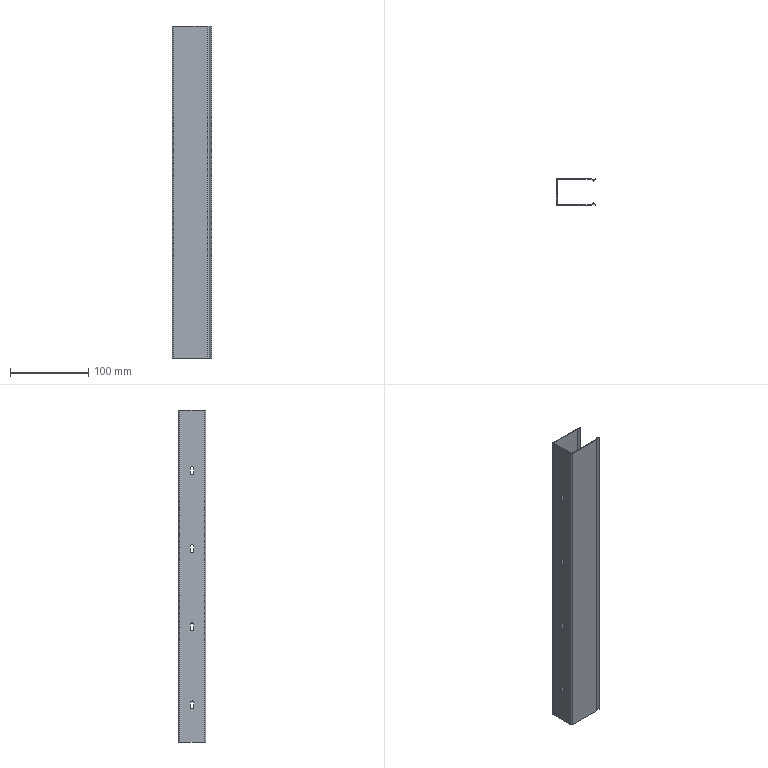Part | STEP file | 35 wire duct_425 | 1 solid | 42 faces | box 50.625 x 35 x 425 mm | volume 57556 mm3 | plane 26 | cylinder 16 | commonest cylinder face diameters 5 x12 1 x2 3 x2